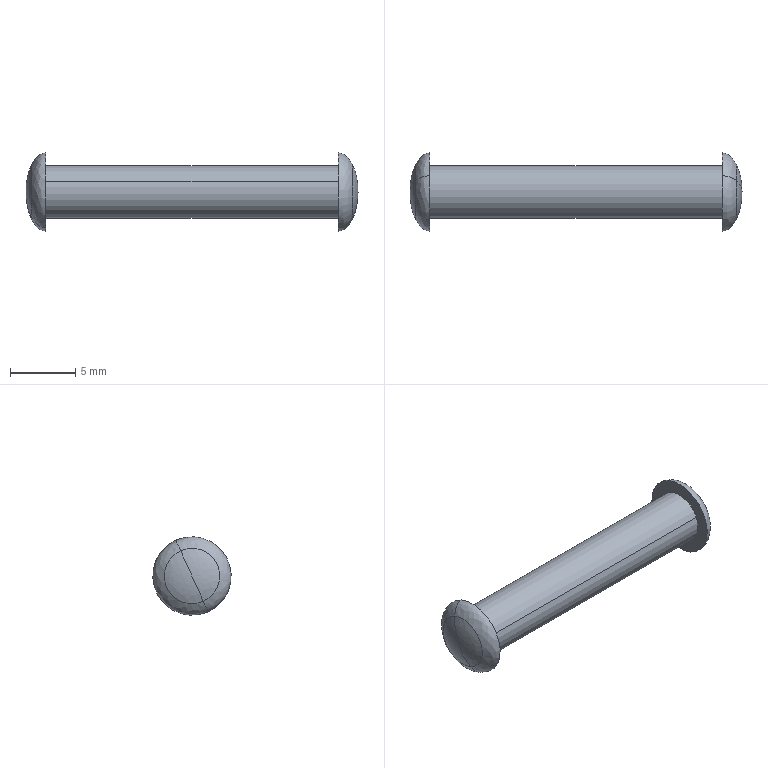Part | STEP file | Component11 | 1 solid | 12 faces | box 25.4 x 6 x 6 mm | volume 338.091 mm3 | spline 8 | cylinder 2 | plane 2 | commonest cylinder face diameters 4 x2
STEP:
#1=CARTESIAN_POINT('',(11.2,19.376,53.32));
#2=VERTEX_POINT('',#1);
#3=CARTESIAN_POINT('',(11.2,23.024,51.68));
#4=VERTEX_POINT('',#3);
#5=CARTESIAN_POINT('',(11.2,21.2,52.5));
#6=DIRECTION('',(1.,0.,0.));
#7=DIRECTION('',(0.,0.9121,-0.4101));
#8=AXIS2_PLACEMENT_3D('',#5,#6,#7);
#9=CIRCLE('',#8,2.);
#10=EDGE_CURVE('',#2,#4,#9,.T.);
#11=ORIENTED_EDGE('',*,*,#10,.F.);
#12=CARTESIAN_POINT('',(-11.2,19.376,53.32));
#13=VERTEX_POINT('',#12);
#14=CARTESIAN_POINT('',(79.567,19.376,53.32));
#15=DIRECTION('',(-1.,0.,0.));
#16=VECTOR('',#15,1000.);
#17=LINE('',#14,#16);
#18=EDGE_CURVE('',#2,#13,#17,.T.);
#19=ORIENTED_EDGE('',*,*,#18,.T.);
#20=CARTESIAN_POINT('',(-11.2,23.024,51.68));
#21=VERTEX_POINT('',#20);
#22=CARTESIAN_POINT('',(-11.2,21.2,52.5));
#23=DIRECTION('',(1.,0.,0.));
#24=DIRECTION('',(0.,0.9121,-0.4101));
#25=AXIS2_PLACEMENT_3D('',#22,#23,#24);
#26=CIRCLE('',#25,2.);
#27=EDGE_CURVE('',#13,#21,#26,.T.);
#28=ORIENTED_EDGE('',*,*,#27,.T.);
#29=CARTESIAN_POINT('',(79.567,23.024,51.68));
#30=DIRECTION('',(-1.,0.,0.));
#31=VECTOR('',#30,1000.);
#32=LINE('',#29,#31);
#33=EDGE_CURVE('',#4,#21,#32,.T.);
#34=ORIENTED_EDGE('',*,*,#33,.F.);
#35=EDGE_LOOP('',(#11,#19,#28,#34));
#36=FACE_OUTER_BOUND('',#35,.T.);
#37=CARTESIAN_POINT('',(79.567,21.2,52.5));
#38=DIRECTION('',(-1.,0.,0.));
#39=DIRECTION('',(0.,0.9121,-0.4101));
#40=AXIS2_PLACEMENT_3D('',#37,#38,#39);
#41=CYLINDRICAL_SURFACE('',#40,2.);
#42=ADVANCED_FACE('',(#36),#41,.T.);
#43=CARTESIAN_POINT('',(-11.2,19.97,49.764));
#44=VERTEX_POINT('',#43);
#45=CARTESIAN_POINT('',(-12.261,20.33,50.565));
#46=VERTEX_POINT('',#45);
#47=CARTESIAN_POINT('',(-11.2,19.97,49.764));
#48=CARTESIAN_POINT('',(-11.603,19.97,49.764));
#49=CARTESIAN_POINT('',(-11.976,20.096,50.045));
#50=CARTESIAN_POINT('',(-12.261,20.33,50.565));
#51=(BOUNDED_CURVE()B_SPLINE_CURVE(3,(#47,#48,#49,#50),.UNSPECIFIED.,.F.,.F.)B_SPLINE_CURVE_WITH_KNOTS((4,4),(3.142,3.927),.UNSPECIFIED.)CURVE()GEOMETRIC_REPRESENTATION_ITEM()RATIONAL_B_SPLINE_CURVE((1.,0.9493,0.9493,1.))REPRESENTATION_ITEM(''));
#52=EDGE_CURVE('',#44,#46,#51,.T.);
#53=ORIENTED_EDGE('',*,*,#52,.T.);
#54=CARTESIAN_POINT('',(-12.261,22.07,54.435));
#55=VERTEX_POINT('',#54);
#56=CARTESIAN_POINT('',(-12.261,21.2,52.5));
#57=DIRECTION('',(1.,0.,0.));
#58=DIRECTION('',(0.,-0.4101,-0.9121));
#59=AXIS2_PLACEMENT_3D('',#56,#57,#58);
#60=CIRCLE('',#59,2.121);
#61=EDGE_CURVE('',#46,#55,#60,.T.);
#62=ORIENTED_EDGE('',*,*,#61,.T.);
#63=CARTESIAN_POINT('',(-11.2,22.43,55.236));
#64=VERTEX_POINT('',#63);
#65=CARTESIAN_POINT('',(-11.2,22.43,55.236));
#66=CARTESIAN_POINT('',(-11.603,22.43,55.236));
#67=CARTESIAN_POINT('',(-11.976,22.304,54.955));
#68=CARTESIAN_POINT('',(-12.261,22.07,54.435));
#69=(BOUNDED_CURVE()B_SPLINE_CURVE(3,(#65,#66,#67,#68),.UNSPECIFIED.,.F.,.F.)B_SPLINE_CURVE_WITH_KNOTS((4,4),(3.142,3.927),.UNSPECIFIED.)CURVE()GEOMETRIC_REPRESENTATION_ITEM()RATIONAL_B_SPLINE_CURVE((1.,0.9493,0.9493,1.))REPRESENTATION_ITEM(''));
#70=EDGE_CURVE('',#64,#55,#69,.T.);
#71=ORIENTED_EDGE('',*,*,#70,.F.);
#72=CARTESIAN_POINT('',(-11.2,21.2,52.5));
#73=DIRECTION('',(1.,0.,0.));
#74=DIRECTION('',(0.,0.9121,-0.4101));
#75=AXIS2_PLACEMENT_3D('',#72,#73,#74);
#76=CIRCLE('',#75,3.);
#77=EDGE_CURVE('',#44,#64,#76,.T.);
#78=ORIENTED_EDGE('',*,*,#77,.F.);
#79=EDGE_LOOP('',(#53,#62,#71,#78));
#80=FACE_OUTER_BOUND('',#79,.T.);
#81=CARTESIAN_POINT('',(-11.2,19.97,49.764));
#82=CARTESIAN_POINT('',(-11.2,22.706,48.534));
#83=CARTESIAN_POINT('',(-11.2,23.936,51.27));
#84=CARTESIAN_POINT('',(-11.2,25.166,54.006));
#85=CARTESIAN_POINT('',(-11.2,22.43,55.236));
#86=CARTESIAN_POINT('',(-12.079,19.97,49.764));
#87=CARTESIAN_POINT('',(-12.079,22.706,48.534));
#88=CARTESIAN_POINT('',(-12.079,23.936,51.27));
#89=CARTESIAN_POINT('',(-12.079,25.166,54.006));
#90=CARTESIAN_POINT('',(-12.079,22.43,55.236));
#91=CARTESIAN_POINT('',(-12.7,20.479,50.897));
#92=CARTESIAN_POINT('',(-12.7,22.082,50.177));
#93=CARTESIAN_POINT('',(-12.7,22.803,51.779));
#94=CARTESIAN_POINT('',(-12.7,23.523,53.382));
#95=CARTESIAN_POINT('',(-12.7,21.921,54.103));
#96=CARTESIAN_POINT('',(-12.7,21.2,52.5));
#97=CARTESIAN_POINT('',(-12.7,21.2,52.5));
#98=CARTESIAN_POINT('',(-12.7,21.2,52.5));
#99=CARTESIAN_POINT('',(-12.7,21.2,52.5));
#100=CARTESIAN_POINT('',(-12.7,21.2,52.5));
#101=(BOUNDED_SURFACE()B_SPLINE_SURFACE(3,2,((#81,#82,#83,#84,#85),(#86,#87,#88,#89,#90),(#91,#92,#93,#94,#95),(#96,#97,#98,#99,#100)),.UNSPECIFIED.,.F.,.F.,.F.)B_SPLINE_SURFACE_WITH_KNOTS((4,4),(3,2,3),(0.,1.),(0.,1.571,3.142),.UNSPECIFIED.)GEOMETRIC_REPRESENTATION_ITEM()RATIONAL_B_SPLINE_SURFACE(((1.,0.7071,1.,0.7071,1.),(0.8047,0.569,0.8047,0.569,0.8047),(0.8047,0.569,0.8047,0.569,0.8047),(1.,0.7071,1.,0.7071,1.)))REPRESENTATION_ITEM('')SURFACE());
#102=ADVANCED_FACE('',(#80),#101,.T.);
#103=CARTESIAN_POINT('',(12.7,21.2,52.5));
#104=VERTEX_POINT('',#103);
#105=CARTESIAN_POINT('',(12.261,20.33,50.565));
#106=VERTEX_POINT('',#105);
#107=CARTESIAN_POINT('',(12.7,21.2,52.5));
#108=CARTESIAN_POINT('',(12.7,20.869,51.765));
#109=CARTESIAN_POINT('',(12.546,20.564,51.085));
#110=CARTESIAN_POINT('',(12.261,20.33,50.565));
#111=(BOUNDED_CURVE()B_SPLINE_CURVE(3,(#107,#108,#109,#110),.UNSPECIFIED.,.F.,.F.)B_SPLINE_CURVE_WITH_KNOTS((4,4),(1.571,2.356),.UNSPECIFIED.)CURVE()GEOMETRIC_REPRESENTATION_ITEM()RATIONAL_B_SPLINE_CURVE((1.,0.9493,0.9493,1.))REPRESENTATION_ITEM(''));
#112=EDGE_CURVE('',#104,#106,#111,.T.);
#113=ORIENTED_EDGE('',*,*,#112,.T.);
#114=CARTESIAN_POINT('',(12.261,22.07,54.435));
#115=VERTEX_POINT('',#114);
#116=CARTESIAN_POINT('',(12.261,21.2,52.5));
#117=DIRECTION('',(1.,0.,0.));
#118=DIRECTION('',(0.,-0.4101,-0.9121));
#119=AXIS2_PLACEMENT_3D('',#116,#117,#118);
#120=CIRCLE('',#119,2.121);
#121=EDGE_CURVE('',#106,#115,#120,.T.);
#122=ORIENTED_EDGE('',*,*,#121,.T.);
#123=CARTESIAN_POINT('',(12.7,21.2,52.5));
#124=CARTESIAN_POINT('',(12.7,21.531,53.235));
#125=CARTESIAN_POINT('',(12.546,21.836,53.915));
#126=CARTESIAN_POINT('',(12.261,22.07,54.435));
#127=(BOUNDED_CURVE()B_SPLINE_CURVE(3,(#123,#124,#125,#126),.UNSPECIFIED.,.F.,.F.)B_SPLINE_CURVE_WITH_KNOTS((4,4),(1.571,2.356),.UNSPECIFIED.)CURVE()GEOMETRIC_REPRESENTATION_ITEM()RATIONAL_B_SPLINE_CURVE((1.,0.9493,0.9493,1.))REPRESENTATION_ITEM(''));
#128=EDGE_CURVE('',#104,#115,#127,.T.);
#129=ORIENTED_EDGE('',*,*,#128,.F.);
#130=EDGE_LOOP('',(#113,#122,#129));
#131=FACE_OUTER_BOUND('',#130,.T.);
#132=CARTESIAN_POINT('',(12.7,21.2,52.5));
#133=CARTESIAN_POINT('',(12.7,21.2,52.5));
#134=CARTESIAN_POINT('',(12.7,21.2,52.5));
#135=CARTESIAN_POINT('',(12.7,21.2,52.5));
#136=CARTESIAN_POINT('',(12.7,21.2,52.5));
#137=CARTESIAN_POINT('',(12.7,20.479,50.897));
#138=CARTESIAN_POINT('',(12.7,22.082,50.177));
#139=CARTESIAN_POINT('',(12.7,22.803,51.779));
#140=CARTESIAN_POINT('',(12.7,23.523,53.382));
#141=CARTESIAN_POINT('',(12.7,21.921,54.103));
#142=CARTESIAN_POINT('',(12.079,19.97,49.764));
#143=CARTESIAN_POINT('',(12.079,22.706,48.534));
#144=CARTESIAN_POINT('',(12.079,23.936,51.27));
#145=CARTESIAN_POINT('',(12.079,25.166,54.006));
#146=CARTESIAN_POINT('',(12.079,22.43,55.236));
#147=CARTESIAN_POINT('',(11.2,19.97,49.764));
#148=CARTESIAN_POINT('',(11.2,22.706,48.534));
#149=CARTESIAN_POINT('',(11.2,23.936,51.27));
#150=CARTESIAN_POINT('',(11.2,25.166,54.006));
#151=CARTESIAN_POINT('',(11.2,22.43,55.236));
#152=(BOUNDED_SURFACE()B_SPLINE_SURFACE(3,2,((#132,#133,#134,#135,#136),(#137,#138,#139,#140,#141),(#142,#143,#144,#145,#146),(#147,#148,#149,#150,#151)),.UNSPECIFIED.,.F.,.F.,.F.)B_SPLINE_SURFACE_WITH_KNOTS((4,4),(3,2,3),(0.,1.),(0.,1.571,3.142),.UNSPECIFIED.)GEOMETRIC_REPRESENTATION_ITEM()RATIONAL_B_SPLINE_SURFACE(((1.,0.7071,1.,0.7071,1.),(0.8047,0.569,0.8047,0.569,0.8047),(0.8047,0.569,0.8047,0.569,0.8047),(1.,0.7071,1.,0.7071,1.)))REPRESENTATION_ITEM('')SURFACE());
#153=ADVANCED_FACE('',(#131),#152,.T.);
#154=ORIENTED_EDGE('',*,*,#128,.T.);
#155=CARTESIAN_POINT('',(12.261,21.2,52.5));
#156=DIRECTION('',(1.,0.,0.));
#157=DIRECTION('',(0.,-0.4101,-0.9121));
#158=AXIS2_PLACEMENT_3D('',#155,#156,#157);
#159=CIRCLE('',#158,2.121);
#160=EDGE_CURVE('',#115,#106,#159,.T.);
#161=ORIENTED_EDGE('',*,*,#160,.T.);
#162=ORIENTED_EDGE('',*,*,#112,.F.);
#163=EDGE_LOOP('',(#154,#161,#162));
#164=FACE_OUTER_BOUND('',#163,.T.);
#165=CARTESIAN_POINT('',(12.7,21.2,52.5));
#166=CARTESIAN_POINT('',(12.7,21.2,52.5));
#167=CARTESIAN_POINT('',(12.7,21.2,52.5));
#168=CARTESIAN_POINT('',(12.7,21.2,52.5));
#169=CARTESIAN_POINT('',(12.7,21.2,52.5));
#170=CARTESIAN_POINT('',(12.7,21.921,54.103));
#171=CARTESIAN_POINT('',(12.7,20.318,54.823));
#172=CARTESIAN_POINT('',(12.7,19.597,53.221));
#173=CARTESIAN_POINT('',(12.7,18.877,51.618));
#174=CARTESIAN_POINT('',(12.7,20.479,50.897));
#175=CARTESIAN_POINT('',(12.079,22.43,55.236));
#176=CARTESIAN_POINT('',(12.079,19.694,56.466));
#177=CARTESIAN_POINT('',(12.079,18.464,53.73));
#178=CARTESIAN_POINT('',(12.079,17.234,50.994));
#179=CARTESIAN_POINT('',(12.079,19.97,49.764));
#180=CARTESIAN_POINT('',(11.2,22.43,55.236));
#181=CARTESIAN_POINT('',(11.2,19.694,56.466));
#182=CARTESIAN_POINT('',(11.2,18.464,53.73));
#183=CARTESIAN_POINT('',(11.2,17.234,50.994));
#184=CARTESIAN_POINT('',(11.2,19.97,49.764));
#185=(BOUNDED_SURFACE()B_SPLINE_SURFACE(3,2,((#165,#166,#167,#168,#169),(#170,#171,#172,#173,#174),(#175,#176,#177,#178,#179),(#180,#181,#182,#183,#184)),.UNSPECIFIED.,.F.,.F.,.F.)B_SPLINE_SURFACE_WITH_KNOTS((4,4),(3,2,3),(0.,1.),(3.142,4.712,6.283),.UNSPECIFIED.)GEOMETRIC_REPRESENTATION_ITEM()RATIONAL_B_SPLINE_SURFACE(((1.,0.7071,1.,0.7071,1.),(0.8047,0.569,0.8047,0.569,0.8047),(0.8047,0.569,0.8047,0.569,0.8047),(1.,0.7071,1.,0.7071,1.)))REPRESENTATION_ITEM('')SURFACE());
#186=ADVANCED_FACE('',(#164),#185,.T.);
#187=ORIENTED_EDGE('',*,*,#70,.T.);
#188=CARTESIAN_POINT('',(-12.261,21.2,52.5));
#189=DIRECTION('',(1.,0.,0.));
#190=DIRECTION('',(0.,-0.4101,-0.9121));
#191=AXIS2_PLACEMENT_3D('',#188,#189,#190);
#192=CIRCLE('',#191,2.121);
#193=EDGE_CURVE('',#55,#46,#192,.T.);
#194=ORIENTED_EDGE('',*,*,#193,.T.);
#195=ORIENTED_EDGE('',*,*,#52,.F.);
#196=CARTESIAN_POINT('',(-11.2,21.2,52.5));
#197=DIRECTION('',(1.,0.,0.));
#198=DIRECTION('',(0.,0.9121,-0.4101));
#199=AXIS2_PLACEMENT_3D('',#196,#197,#198);
#200=CIRCLE('',#199,3.);
#201=EDGE_CURVE('',#64,#44,#200,.T.);
#202=ORIENTED_EDGE('',*,*,#201,.F.);
#203=EDGE_LOOP('',(#187,#194,#195,#202));
#204=FACE_OUTER_BOUND('',#203,.T.);
#205=CARTESIAN_POINT('',(-11.2,22.43,55.236));
#206=CARTESIAN_POINT('',(-11.2,19.694,56.466));
#207=CARTESIAN_POINT('',(-11.2,18.464,53.73));
#208=CARTESIAN_POINT('',(-11.2,17.234,50.994));
#209=CARTESIAN_POINT('',(-11.2,19.97,49.764));
#210=CARTESIAN_POINT('',(-12.079,22.43,55.236));
#211=CARTESIAN_POINT('',(-12.079,19.694,56.466));
#212=CARTESIAN_POINT('',(-12.079,18.464,53.73));
#213=CARTESIAN_POINT('',(-12.079,17.234,50.994));
#214=CARTESIAN_POINT('',(-12.079,19.97,49.764));
#215=CARTESIAN_POINT('',(-12.7,21.921,54.103));
#216=CARTESIAN_POINT('',(-12.7,20.318,54.823));
#217=CARTESIAN_POINT('',(-12.7,19.597,53.221));
#218=CARTESIAN_POINT('',(-12.7,18.877,51.618));
#219=CARTESIAN_POINT('',(-12.7,20.479,50.897));
#220=CARTESIAN_POINT('',(-12.7,21.2,52.5));
#221=CARTESIAN_POINT('',(-12.7,21.2,52.5));
#222=CARTESIAN_POINT('',(-12.7,21.2,52.5));
#223=CARTESIAN_POINT('',(-12.7,21.2,52.5));
#224=CARTESIAN_POINT('',(-12.7,21.2,52.5));
#225=(BOUNDED_SURFACE()B_SPLINE_SURFACE(3,2,((#205,#206,#207,#208,#209),(#210,#211,#212,#213,#214),(#215,#216,#217,#218,#219),(#220,#221,#222,#223,#224)),.UNSPECIFIED.,.F.,.F.,.F.)B_SPLINE_SURFACE_WITH_KNOTS((4,4),(3,2,3),(0.,1.),(3.142,4.712,6.283),.UNSPECIFIED.)GEOMETRIC_REPRESENTATION_ITEM()RATIONAL_B_SPLINE_SURFACE(((1.,0.7071,1.,0.7071,1.),(0.8047,0.569,0.8047,0.569,0.8047),(0.8047,0.569,0.8047,0.569,0.8047),(1.,0.7071,1.,0.7071,1.)))REPRESENTATION_ITEM('')SURFACE());
#226=ADVANCED_FACE('',(#204),#225,.T.);
#227=ORIENTED_EDGE('',*,*,#193,.F.);
#228=CARTESIAN_POINT('',(-12.7,21.2,52.5));
#229=VERTEX_POINT('',#228);
#230=CARTESIAN_POINT('',(-12.261,22.07,54.435));
#231=CARTESIAN_POINT('',(-12.546,21.836,53.915));
#232=CARTESIAN_POINT('',(-12.7,21.531,53.235));
#233=CARTESIAN_POINT('',(-12.7,21.2,52.5));
#234=(BOUNDED_CURVE()B_SPLINE_CURVE(3,(#230,#231,#232,#233),.UNSPECIFIED.,.F.,.F.)B_SPLINE_CURVE_WITH_KNOTS((4,4),(3.927,4.712),.UNSPECIFIED.)CURVE()GEOMETRIC_REPRESENTATION_ITEM()RATIONAL_B_SPLINE_CURVE((1.,0.9493,0.9493,1.))REPRESENTATION_ITEM(''));
#235=EDGE_CURVE('',#55,#229,#234,.T.);
#236=ORIENTED_EDGE('',*,*,#235,.T.);
#237=CARTESIAN_POINT('',(-12.261,20.33,50.565));
#238=CARTESIAN_POINT('',(-12.546,20.564,51.085));
#239=CARTESIAN_POINT('',(-12.7,20.869,51.765));
#240=CARTESIAN_POINT('',(-12.7,21.2,52.5));
#241=(BOUNDED_CURVE()B_SPLINE_CURVE(3,(#237,#238,#239,#240),.UNSPECIFIED.,.F.,.F.)B_SPLINE_CURVE_WITH_KNOTS((4,4),(3.927,4.712),.UNSPECIFIED.)CURVE()GEOMETRIC_REPRESENTATION_ITEM()RATIONAL_B_SPLINE_CURVE((1.,0.9493,0.9493,1.))REPRESENTATION_ITEM(''));
#242=EDGE_CURVE('',#46,#229,#241,.T.);
#243=ORIENTED_EDGE('',*,*,#242,.F.);
#244=EDGE_LOOP('',(#227,#236,#243));
#245=FACE_OUTER_BOUND('',#244,.T.);
#246=CARTESIAN_POINT('',(-11.2,22.43,55.236));
#247=CARTESIAN_POINT('',(-11.2,19.694,56.466));
#248=CARTESIAN_POINT('',(-11.2,18.464,53.73));
#249=CARTESIAN_POINT('',(-11.2,17.234,50.994));
#250=CARTESIAN_POINT('',(-11.2,19.97,49.764));
#251=CARTESIAN_POINT('',(-12.079,22.43,55.236));
#252=CARTESIAN_POINT('',(-12.079,19.694,56.466));
#253=CARTESIAN_POINT('',(-12.079,18.464,53.73));
#254=CARTESIAN_POINT('',(-12.079,17.234,50.994));
#255=CARTESIAN_POINT('',(-12.079,19.97,49.764));
#256=CARTESIAN_POINT('',(-12.7,21.921,54.103));
#257=CARTESIAN_POINT('',(-12.7,20.318,54.823));
#258=CARTESIAN_POINT('',(-12.7,19.597,53.221));
#259=CARTESIAN_POINT('',(-12.7,18.877,51.618));
#260=CARTESIAN_POINT('',(-12.7,20.479,50.897));
#261=CARTESIAN_POINT('',(-12.7,21.2,52.5));
#262=CARTESIAN_POINT('',(-12.7,21.2,52.5));
#263=CARTESIAN_POINT('',(-12.7,21.2,52.5));
#264=CARTESIAN_POINT('',(-12.7,21.2,52.5));
#265=CARTESIAN_POINT('',(-12.7,21.2,52.5));
#266=(BOUNDED_SURFACE()B_SPLINE_SURFACE(3,2,((#246,#247,#248,#249,#250),(#251,#252,#253,#254,#255),(#256,#257,#258,#259,#260),(#261,#262,#263,#264,#265)),.UNSPECIFIED.,.F.,.F.,.F.)B_SPLINE_SURFACE_WITH_KNOTS((4,4),(3,2,3),(0.,1.),(3.142,4.712,6.283),.UNSPECIFIED.)GEOMETRIC_REPRESENTATION_ITEM()RATIONAL_B_SPLINE_SURFACE(((1.,0.7071,1.,0.7071,1.),(0.8047,0.569,0.8047,0.569,0.8047),(0.8047,0.569,0.8047,0.569,0.8047),(1.,0.7071,1.,0.7071,1.)))REPRESENTATION_ITEM('')SURFACE());
#267=ADVANCED_FACE('',(#245),#266,.T.);
#268=ORIENTED_EDGE('',*,*,#160,.F.);
#269=CARTESIAN_POINT('',(11.2,22.43,55.236));
#270=VERTEX_POINT('',#269);
#271=CARTESIAN_POINT('',(12.261,22.07,54.435));
#272=CARTESIAN_POINT('',(11.976,22.304,54.955));
#273=CARTESIAN_POINT('',(11.603,22.43,55.236));
#274=CARTESIAN_POINT('',(11.2,22.43,55.236));
#275=(BOUNDED_CURVE()B_SPLINE_CURVE(3,(#271,#272,#273,#274),.UNSPECIFIED.,.F.,.F.)B_SPLINE_CURVE_WITH_KNOTS((4,4),(2.356,3.142),.UNSPECIFIED.)CURVE()GEOMETRIC_REPRESENTATION_ITEM()RATIONAL_B_SPLINE_CURVE((1.,0.9493,0.9493,1.))REPRESENTATION_ITEM(''));
#276=EDGE_CURVE('',#115,#270,#275,.T.);
#277=ORIENTED_EDGE('',*,*,#276,.T.);
#278=CARTESIAN_POINT('',(11.2,19.97,49.764));
#279=VERTEX_POINT('',#278);
#280=CARTESIAN_POINT('',(11.2,21.2,52.5));
#281=DIRECTION('',(1.,0.,0.));
#282=DIRECTION('',(0.,0.9121,-0.4101));
#283=AXIS2_PLACEMENT_3D('',#280,#281,#282);
#284=CIRCLE('',#283,3.);
#285=EDGE_CURVE('',#270,#279,#284,.T.);
#286=ORIENTED_EDGE('',*,*,#285,.T.);
#287=CARTESIAN_POINT('',(12.261,20.33,50.565));
#288=CARTESIAN_POINT('',(11.976,20.096,50.045));
#289=CARTESIAN_POINT('',(11.603,19.97,49.764));
#290=CARTESIAN_POINT('',(11.2,19.97,49.764));
#291=(BOUNDED_CURVE()B_SPLINE_CURVE(3,(#287,#288,#289,#290),.UNSPECIFIED.,.F.,.F.)B_SPLINE_CURVE_WITH_KNOTS((4,4),(2.356,3.142),.UNSPECIFIED.)CURVE()GEOMETRIC_REPRESENTATION_ITEM()RATIONAL_B_SPLINE_CURVE((1.,0.9493,0.9493,1.))REPRESENTATION_ITEM(''));
#292=EDGE_CURVE('',#106,#279,#291,.T.);
#293=ORIENTED_EDGE('',*,*,#292,.F.);
#294=EDGE_LOOP('',(#268,#277,#286,#293));
#295=FACE_OUTER_BOUND('',#294,.T.);
#296=CARTESIAN_POINT('',(12.7,21.2,52.5));
#297=CARTESIAN_POINT('',(12.7,21.2,52.5));
#298=CARTESIAN_POINT('',(12.7,21.2,52.5));
#299=CARTESIAN_POINT('',(12.7,21.2,52.5));
#300=CARTESIAN_POINT('',(12.7,21.2,52.5));
#301=CARTESIAN_POINT('',(12.7,21.921,54.103));
#302=CARTESIAN_POINT('',(12.7,20.318,54.823));
#303=CARTESIAN_POINT('',(12.7,19.597,53.221));
#304=CARTESIAN_POINT('',(12.7,18.877,51.618));
#305=CARTESIAN_POINT('',(12.7,20.479,50.897));
#306=CARTESIAN_POINT('',(12.079,22.43,55.236));
#307=CARTESIAN_POINT('',(12.079,19.694,56.466));
#308=CARTESIAN_POINT('',(12.079,18.464,53.73));
#309=CARTESIAN_POINT('',(12.079,17.234,50.994));
#310=CARTESIAN_POINT('',(12.079,19.97,49.764));
#311=CARTESIAN_POINT('',(11.2,22.43,55.236));
#312=CARTESIAN_POINT('',(11.2,19.694,56.466));
#313=CARTESIAN_POINT('',(11.2,18.464,53.73));
#314=CARTESIAN_POINT('',(11.2,17.234,50.994));
#315=CARTESIAN_POINT('',(11.2,19.97,49.764));
#316=(BOUNDED_SURFACE()B_SPLINE_SURFACE(3,2,((#296,#297,#298,#299,#300),(#301,#302,#303,#304,#305),(#306,#307,#308,#309,#310),(#311,#312,#313,#314,#315)),.UNSPECIFIED.,.F.,.F.,.F.)B_SPLINE_SURFACE_WITH_KNOTS((4,4),(3,2,3),(0.,1.),(3.142,4.712,6.283),.UNSPECIFIED.)GEOMETRIC_REPRESENTATION_ITEM()RATIONAL_B_SPLINE_SURFACE(((1.,0.7071,1.,0.7071,1.),(0.8047,0.569,0.8047,0.569,0.8047),(0.8047,0.569,0.8047,0.569,0.8047),(1.,0.7071,1.,0.7071,1.)))REPRESENTATION_ITEM('')SURFACE());
#317=ADVANCED_FACE('',(#295),#316,.T.);
#318=ORIENTED_EDGE('',*,*,#121,.F.);
#319=ORIENTED_EDGE('',*,*,#292,.T.);
#320=CARTESIAN_POINT('',(11.2,21.2,52.5));
#321=DIRECTION('',(1.,0.,0.));
#322=DIRECTION('',(0.,0.9121,-0.4101));
#323=AXIS2_PLACEMENT_3D('',#320,#321,#322);
#324=CIRCLE('',#323,3.);
#325=EDGE_CURVE('',#279,#270,#324,.T.);
#326=ORIENTED_EDGE('',*,*,#325,.T.);
#327=ORIENTED_EDGE('',*,*,#276,.F.);
#328=EDGE_LOOP('',(#318,#319,#326,#327));
#329=FACE_OUTER_BOUND('',#328,.T.);
#330=CARTESIAN_POINT('',(12.7,21.2,52.5));
#331=CARTESIAN_POINT('',(12.7,21.2,52.5));
#332=CARTESIAN_POINT('',(12.7,21.2,52.5));
#333=CARTESIAN_POINT('',(12.7,21.2,52.5));
#334=CARTESIAN_POINT('',(12.7,21.2,52.5));
#335=CARTESIAN_POINT('',(12.7,20.479,50.897));
#336=CARTESIAN_POINT('',(12.7,22.082,50.177));
#337=CARTESIAN_POINT('',(12.7,22.803,51.779));
#338=CARTESIAN_POINT('',(12.7,23.523,53.382));
#339=CARTESIAN_POINT('',(12.7,21.921,54.103));
#340=CARTESIAN_POINT('',(12.079,19.97,49.764));
#341=CARTESIAN_POINT('',(12.079,22.706,48.534));
#342=CARTESIAN_POINT('',(12.079,23.936,51.27));
#343=CARTESIAN_POINT('',(12.079,25.166,54.006));
#344=CARTESIAN_POINT('',(12.079,22.43,55.236));
#345=CARTESIAN_POINT('',(11.2,19.97,49.764));
#346=CARTESIAN_POINT('',(11.2,22.706,48.534));
#347=CARTESIAN_POINT('',(11.2,23.936,51.27));
#348=CARTESIAN_POINT('',(11.2,25.166,54.006));
#349=CARTESIAN_POINT('',(11.2,22.43,55.236));
#350=(BOUNDED_SURFACE()B_SPLINE_SURFACE(3,2,((#330,#331,#332,#333,#334),(#335,#336,#337,#338,#339),(#340,#341,#342,#343,#344),(#345,#346,#347,#348,#349)),.UNSPECIFIED.,.F.,.F.,.F.)B_SPLINE_SURFACE_WITH_KNOTS((4,4),(3,2,3),(0.,1.),(0.,1.571,3.142),.UNSPECIFIED.)GEOMETRIC_REPRESENTATION_ITEM()RATIONAL_B_SPLINE_SURFACE(((1.,0.7071,1.,0.7071,1.),(0.8047,0.569,0.8047,0.569,0.8047),(0.8047,0.569,0.8047,0.569,0.8047),(1.,0.7071,1.,0.7071,1.)))REPRESENTATION_ITEM('')SURFACE());
#351=ADVANCED_FACE('',(#329),#350,.T.);
#352=CARTESIAN_POINT('',(11.2,21.2,52.5));
#353=DIRECTION('',(1.,0.,0.));
#354=DIRECTION('',(0.,0.9121,-0.4101));
#355=AXIS2_PLACEMENT_3D('',#352,#353,#354);
#356=CIRCLE('',#355,2.);
#357=EDGE_CURVE('',#4,#2,#356,.T.);
#358=ORIENTED_EDGE('',*,*,#357,.T.);
#359=ORIENTED_EDGE('',*,*,#10,.T.);
#360=EDGE_LOOP('',(#358,#359));
#361=FACE_BOUND('',#360,.T.);
#362=ORIENTED_EDGE('',*,*,#325,.F.);
#363=ORIENTED_EDGE('',*,*,#285,.F.);
#364=EDGE_LOOP('',(#362,#363));
#365=FACE_OUTER_BOUND('',#364,.T.);
#366=CARTESIAN_POINT('',(11.2,19.955,49.731));
#367=DIRECTION('',(-1.,0.,0.));
#368=DIRECTION('',(0.,0.,1.));
#369=AXIS2_PLACEMENT_3D('',#366,#367,#368);
#370=PLANE('',#369);
#371=ADVANCED_FACE('',(#361,#365),#370,.T.);
#372=CARTESIAN_POINT('',(-11.2,21.2,52.5));
#373=DIRECTION('',(1.,0.,0.));
#374=DIRECTION('',(0.,0.9121,-0.4101));
#375=AXIS2_PLACEMENT_3D('',#372,#373,#374);
#376=CIRCLE('',#375,2.);
#377=EDGE_CURVE('',#21,#13,#376,.T.);
#378=ORIENTED_EDGE('',*,*,#377,.F.);
#379=ORIENTED_EDGE('',*,*,#27,.F.);
#380=EDGE_LOOP('',(#378,#379));
#381=FACE_BOUND('',#380,.T.);
#382=ORIENTED_EDGE('',*,*,#77,.T.);
#383=ORIENTED_EDGE('',*,*,#201,.T.);
#384=EDGE_LOOP('',(#382,#383));
#385=FACE_OUTER_BOUND('',#384,.T.);
#386=CARTESIAN_POINT('',(-11.2,19.955,49.731));
#387=DIRECTION('',(1.,0.,0.));
#388=DIRECTION('',(0.,1.,0.));
#389=AXIS2_PLACEMENT_3D('',#386,#387,#388);
#390=PLANE('',#389);
#391=ADVANCED_FACE('',(#381,#385),#390,.T.);
#392=ORIENTED_EDGE('',*,*,#18,.F.);
#393=ORIENTED_EDGE('',*,*,#357,.F.);
#394=ORIENTED_EDGE('',*,*,#33,.T.);
#395=ORIENTED_EDGE('',*,*,#377,.T.);
#396=EDGE_LOOP('',(#392,#393,#394,#395));
#397=FACE_OUTER_BOUND('',#396,.T.);
#398=CARTESIAN_POINT('',(79.567,21.2,52.5));
#399=DIRECTION('',(-1.,0.,0.));
#400=DIRECTION('',(0.,0.9121,-0.4101));
#401=AXIS2_PLACEMENT_3D('',#398,#399,#400);
#402=CYLINDRICAL_SURFACE('',#401,2.);
#403=ADVANCED_FACE('',(#397),#402,.T.);
#404=ORIENTED_EDGE('',*,*,#61,.F.);
#405=ORIENTED_EDGE('',*,*,#242,.T.);
#406=ORIENTED_EDGE('',*,*,#235,.F.);
#407=EDGE_LOOP('',(#404,#405,#406));
#408=FACE_OUTER_BOUND('',#407,.T.);
#409=CARTESIAN_POINT('',(-11.2,19.97,49.764));
#410=CARTESIAN_POINT('',(-11.2,22.706,48.534));
#411=CARTESIAN_POINT('',(-11.2,23.936,51.27));
#412=CARTESIAN_POINT('',(-11.2,25.166,54.006));
#413=CARTESIAN_POINT('',(-11.2,22.43,55.236));
#414=CARTESIAN_POINT('',(-12.079,19.97,49.764));
#415=CARTESIAN_POINT('',(-12.079,22.706,48.534));
#416=CARTESIAN_POINT('',(-12.079,23.936,51.27));
#417=CARTESIAN_POINT('',(-12.079,25.166,54.006));
#418=CARTESIAN_POINT('',(-12.079,22.43,55.236));
#419=CARTESIAN_POINT('',(-12.7,20.479,50.897));
#420=CARTESIAN_POINT('',(-12.7,22.082,50.177));
#421=CARTESIAN_POINT('',(-12.7,22.803,51.779));
#422=CARTESIAN_POINT('',(-12.7,23.523,53.382));
#423=CARTESIAN_POINT('',(-12.7,21.921,54.103));
#424=CARTESIAN_POINT('',(-12.7,21.2,52.5));
#425=CARTESIAN_POINT('',(-12.7,21.2,52.5));
#426=CARTESIAN_POINT('',(-12.7,21.2,52.5));
#427=CARTESIAN_POINT('',(-12.7,21.2,52.5));
#428=CARTESIAN_POINT('',(-12.7,21.2,52.5));
#429=(BOUNDED_SURFACE()B_SPLINE_SURFACE(3,2,((#409,#410,#411,#412,#413),(#414,#415,#416,#417,#418),(#419,#420,#421,#422,#423),(#424,#425,#426,#427,#428)),.UNSPECIFIED.,.F.,.F.,.F.)B_SPLINE_SURFACE_WITH_KNOTS((4,4),(3,2,3),(0.,1.),(0.,1.571,3.142),.UNSPECIFIED.)GEOMETRIC_REPRESENTATION_ITEM()RATIONAL_B_SPLINE_SURFACE(((1.,0.7071,1.,0.7071,1.),(0.8047,0.569,0.8047,0.569,0.8047),(0.8047,0.569,0.8047,0.569,0.8047),(1.,0.7071,1.,0.7071,1.)))REPRESENTATION_ITEM('')SURFACE());
#430=ADVANCED_FACE('',(#408),#429,.T.);
#431=CLOSED_SHELL('',(#42,#102,#153,#186,#226,#267,#317,#351,#371,#391,#403,#430));
#432=MANIFOLD_SOLID_BREP('',#431);
#433=CARTESIAN_POINT('',(0.,0.,0.));
#434=DIRECTION('',(0.,0.,1.));
#435=DIRECTION('',(1.,0.,0.));
#436=AXIS2_PLACEMENT_3D('',#433,#434,#435);
#437=(LENGTH_UNIT()NAMED_UNIT(*)SI_UNIT(.MILLI.,.METRE.));
#438=UNCERTAINTY_MEASURE_WITH_UNIT(LENGTH_MEASURE(0.00001),#437,'','');
#439=(NAMED_UNIT(*)PLANE_ANGLE_UNIT()SI_UNIT($,.RADIAN.));
#440=(NAMED_UNIT(*)SI_UNIT($,.STERADIAN.)SOLID_ANGLE_UNIT());
#441=(GEOMETRIC_REPRESENTATION_CONTEXT(3)GLOBAL_UNCERTAINTY_ASSIGNED_CONTEXT((#438))GLOBAL_UNIT_ASSIGNED_CONTEXT((#437,#439,#440))REPRESENTATION_CONTEXT('',''));
#442=ADVANCED_BREP_SHAPE_REPRESENTATION('',(#432,#436),#441);